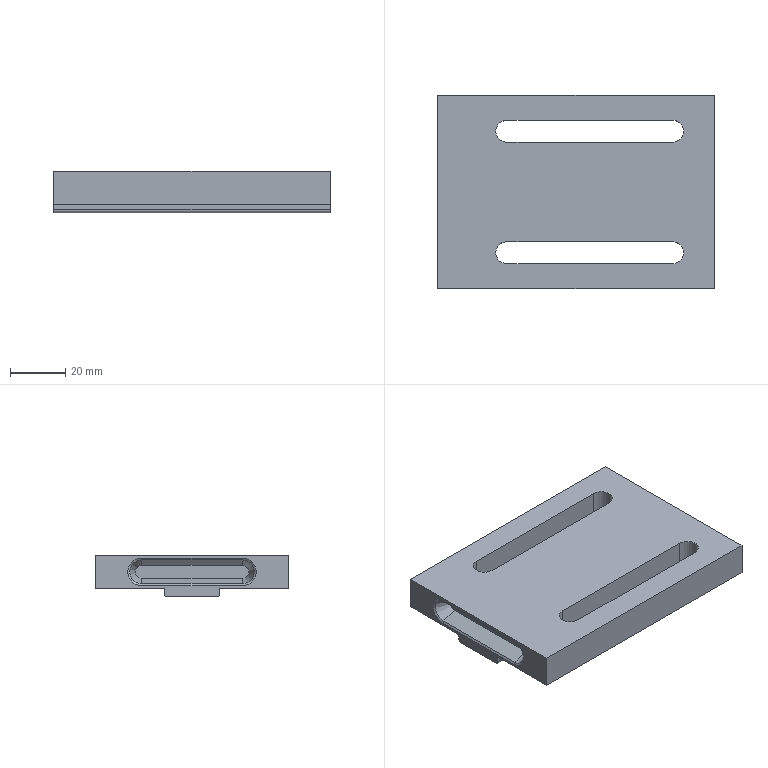Part | STEP file | Tube necking machine_id434_x_t | 1 solid | 29 faces | box 100 x 70 x 15 mm | volume 75500 mm3 | plane 19 | cylinder 6 | cone 4 | commonest cylinder face diameters 8 x4 2 x2